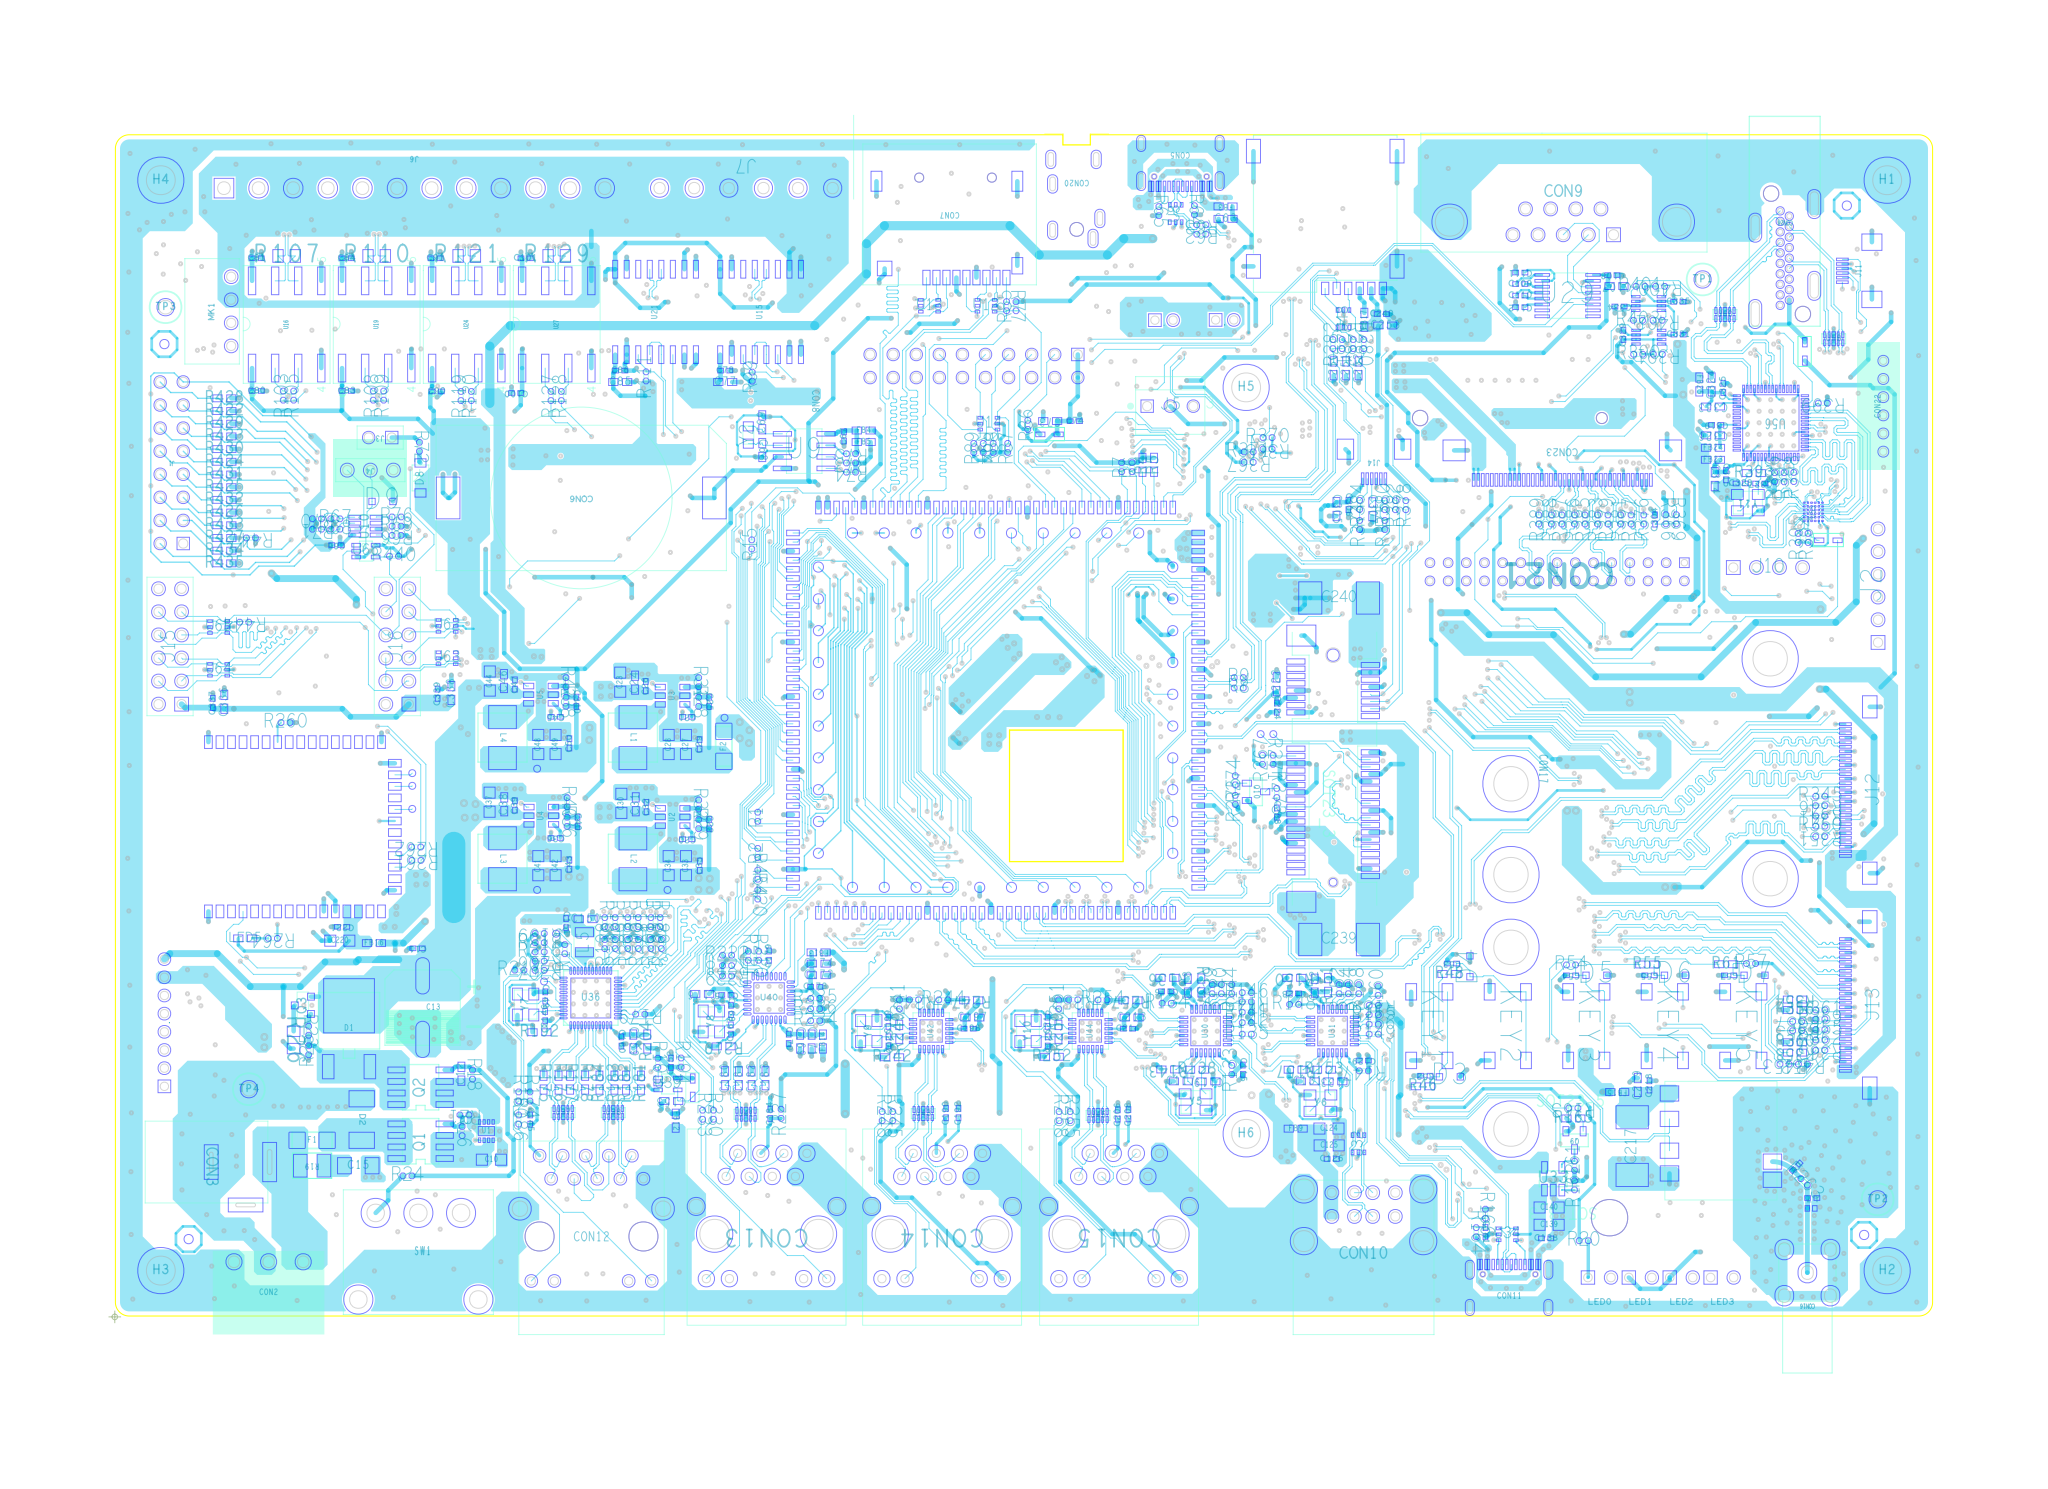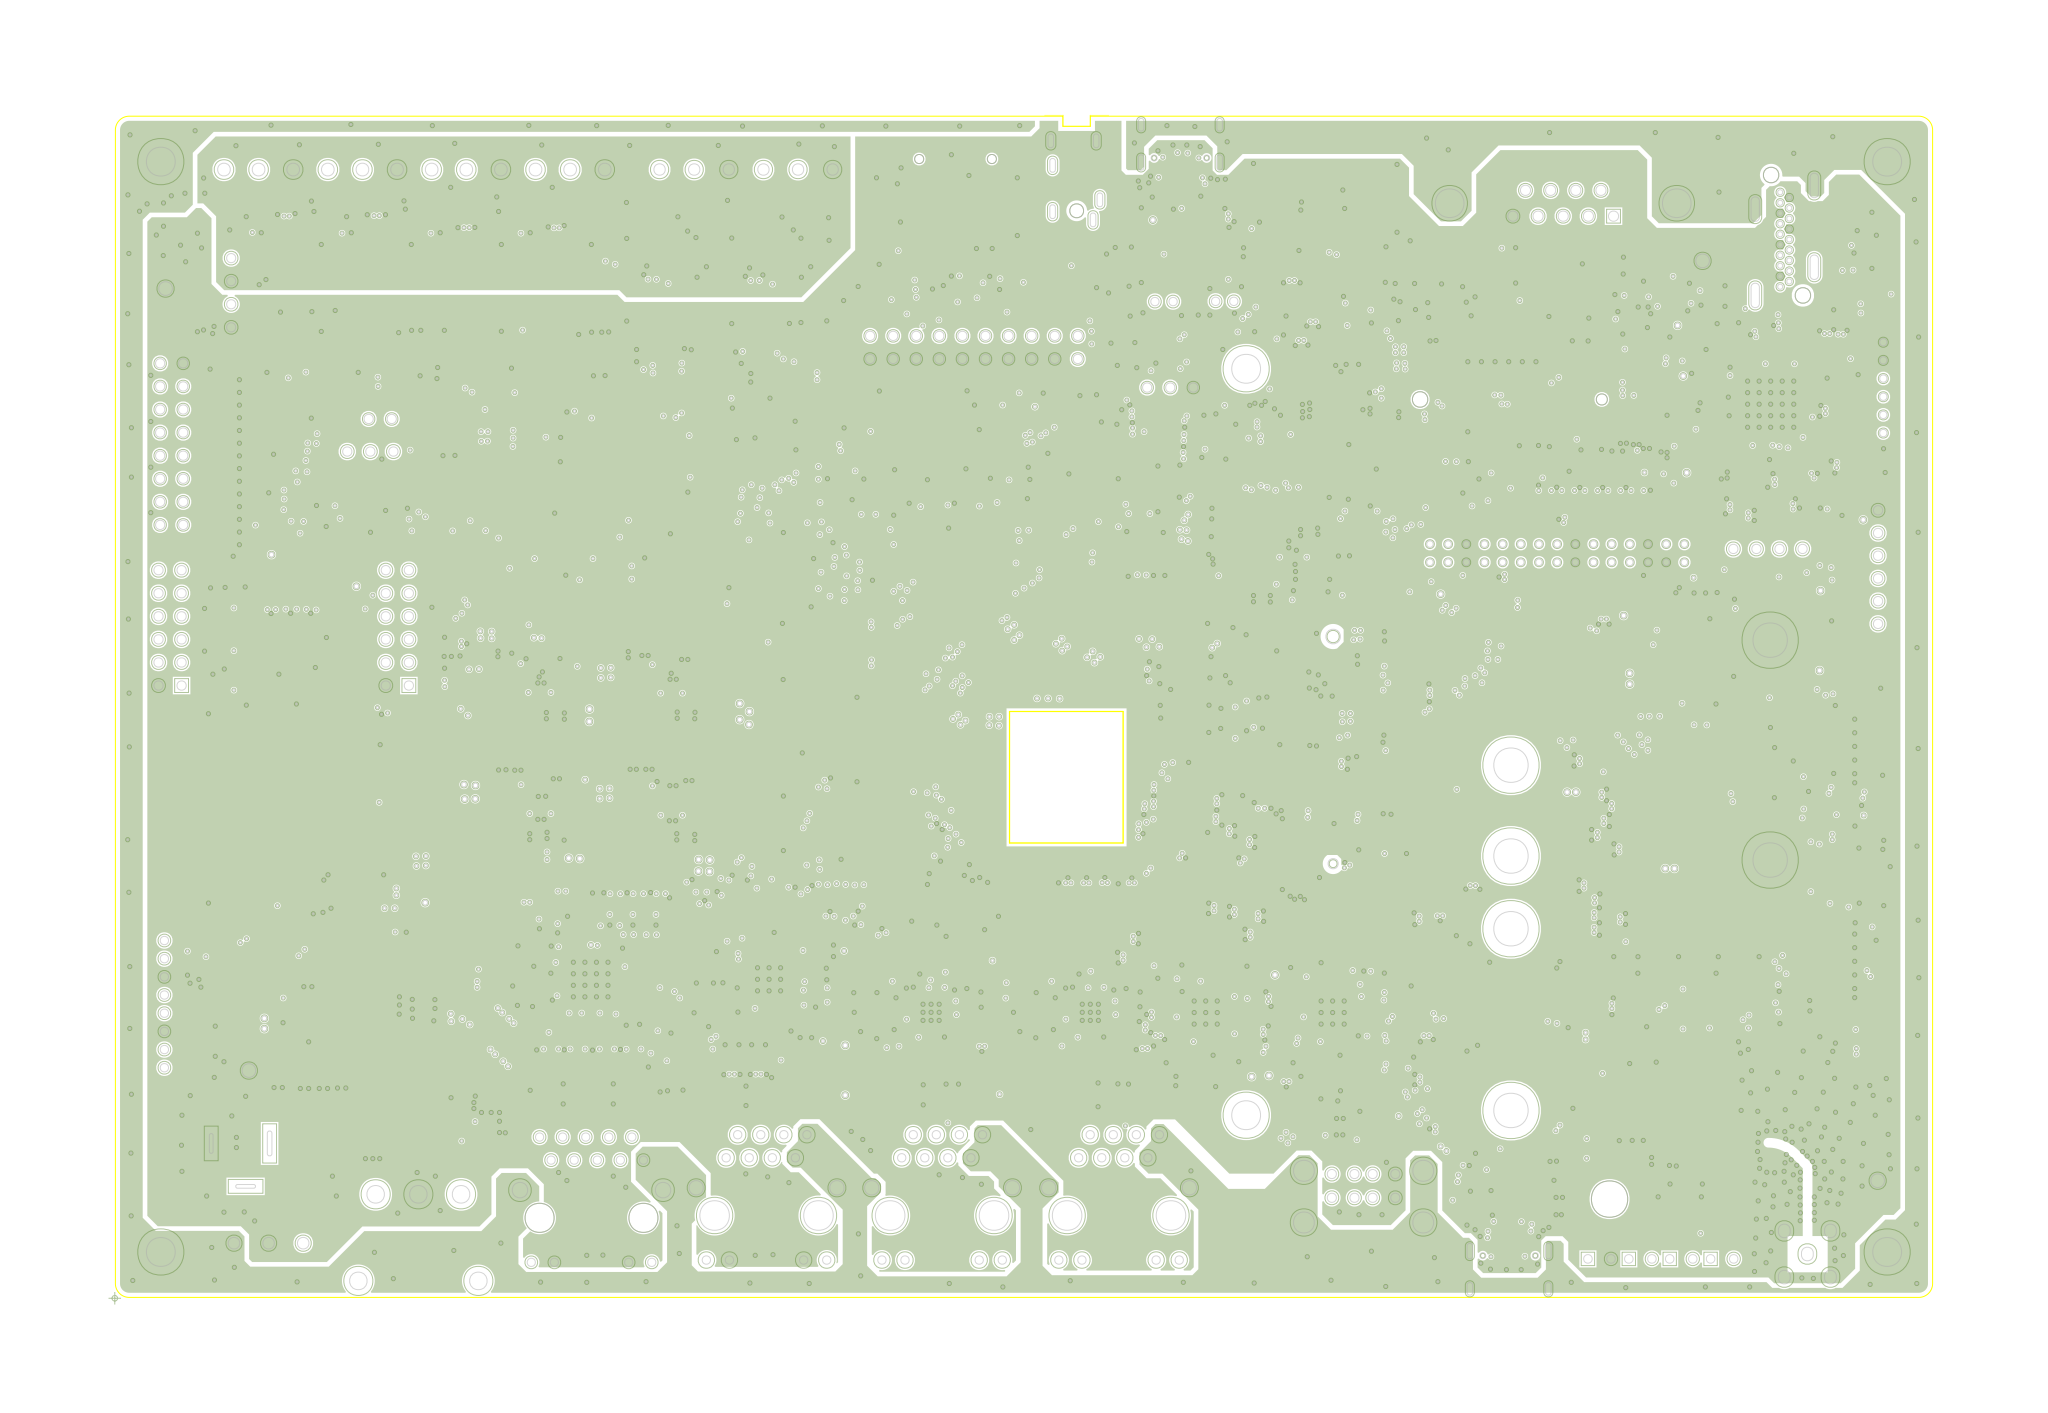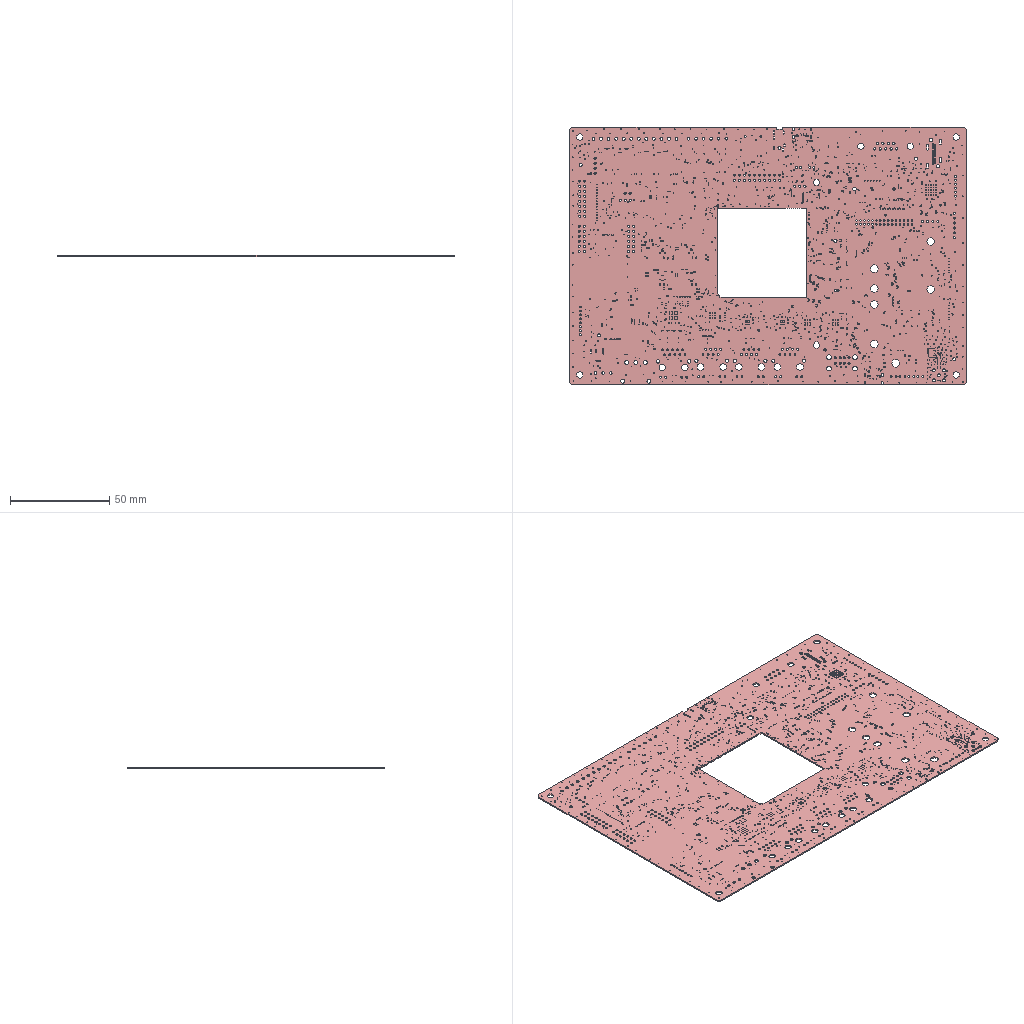Circuit board layout | Cadence Allegro | box 200 x 130 x 0.7 mm
Layer stack:
# Cadence Allegro layer stack of  (unit mm; from the constraint file cross-section; dielectric type: 0 not recorded (Allegro does not mark core vs prepreg), 3 surface material)
index,name,kind,layer,copper_thickness_mm,dielectric_type,dielectric_thickness_mm,dielectric_material,dielectric_constant
0,Top Surface,other,,,,,,
1,TOP,copper,TOP,0.0305,,,,
2,Dielectric1,dielectric,,,0,0.2032,FR-4,4.5
3,GND02,copper,GND02,0.0305,,,,
4,Dielectric2,dielectric,,,0,0.2032,FR-4,4.5
5,VCC03,copper,VCC03,0.0305,,,,
6,Dielectric3,dielectric,,,0,0.2032,FR-4,4.5
7,BOTTOM,copper,BOTTOM,0.0305,,,,
8,Bottom Surface,other,,,,,,
# drill layer pairs: low layer,high layer
drill_pair,TOP,BOTTOM
Part placement, first 484 of 1029 lines:
REFDES,COMP_VALUE,SYM_NAME,SYM_X,SYM_Y,SYM_ROTATE,SYM_MIRROR
C1,680pF_50V,C0603,4512.00,3287.50,180.000,YES
C2,680pF_50V,C0603,4392.00,3287.50,0.000,YES
C3,100nF_25V,C0402,3314.00,3524.00,0.000,YES
C4,100nF_25V,C0402,3314.00,3480.00,0.000,YES
C5,22uF_25V,C0805,4771.35,3338.00,0.000,YES
C6,22uF_25V,C0805,4771.35,3263.00,0.000,YES
C7,100nF_25V,C0402,4707.00,3397.00,180.000,YES
C8,33pF_50V,C0603,3205.00,3430.50,0.000,YES
C9,33pF_50V,C0603,3328.00,3430.50,180.000,YES
C10,22uF_25V,C0805,1590.65,681.00,0.000,NO
C11,100nF_25V,C0402,1312.00,1597.00,180.000,NO
C12,1uF_25V,C0603,1501.88,1053.48,90.000,NO
C13,220uF_35V,CAP_ALU_SMD_8X10D5,1333.90,1340.00,0.000,NO
C14,22pF_50V,C0603,1524.50,805.00,90.000,YES
C15,2.2uF_25V,C1206,1055.00,655.00,0.000,NO
C16,10uF_25V,C0603,364.50,1450.00,90.000,YES
C17,100nF_25V,C0402,315.00,1455.00,90.000,YES
C18,10uF_25V,C0603,316.50,1299.00,270.000,YES
C19,100nF_25V,C0402,366.00,1299.00,270.000,YES
C20,100nF_25V,C0402,2480.00,2070.00,180.000,NO
C21,100nF_25V,C0402,2480.00,2600.00,180.000,NO
C22,15pF_50V,C0402,2575.00,2135.00,270.000,NO
C23,22uF_25V,C0805,2190.00,2708.65,90.000,NO
C24,1uF_25V,C0603,2254.50,2748.00,90.000,NO
C25,15pF_50V,C0402,2575.00,2665.00,270.000,NO
C26,100nF_25V,C0402,2301.00,2733.00,90.000,NO
C27,22uF_25V,C0805,2475.00,2438.65,90.000,NO
C28,22uF_25V,C0805,2400.00,2438.65,90.000,NO
C29,100nF_25V,C0402,2534.00,2481.00,90.000,NO
C30,22uF_25V,C0805,2195.00,2183.65,90.000,NO
C31,1uF_25V,C0603,2257.50,2221.00,90.000,NO
C32,100nF_25V,C0402,2304.00,2209.00,90.000,NO
C33,22uF_25V,C0805,2475.00,1913.66,90.000,NO
C34,22uF_25V,C0805,2400.00,1913.65,90.000,NO
C35,100nF_25V,C0402,2535.00,1955.00,90.000,NO
C36,100nF_25V,C0402,1909.99,2075.00,180.000,NO
C37,22uF_25V,C0805,1623.99,2188.65,90.000,NO
C38,1uF_25V,C0603,1687.49,2221.00,90.000,NO
C39,100nF_25V,C0402,1733.99,2216.00,90.000,NO
C40,15pF_50V,C0402,2004.99,2145.00,270.000,NO
C41,22uF_25V,C0805,1834.99,1913.65,90.000,NO
C42,22uF_25V,C0805,1909.99,1913.65,90.000,NO
C43,100nF_25V,C0402,1969.99,1960.00,90.000,NO
C44,22uF_25V,C0805,1625.00,2713.65,90.000,NO
C45,100nF_25V,C0402,1910.00,2600.00,180.000,NO
C46,1uF_25V,C0603,1686.50,2755.00,90.000,NO
C47,100nF_25V,C0402,1734.00,2740.00,90.000,NO
C48,22uF_25V,C0805,1835.00,2438.65,90.000,NO
C49,22uF_25V,C0805,1910.00,2438.66,90.000,NO
C50,100nF_25V,C0402,1970.00,2485.00,90.000,NO
C51,1nF_2KV,C1210,285.00,4670.00,90.000,YES
C52,10nF_50V,C0402,5679.00,1045.00,180.000,NO
C53,10nF_50V,C0402,5794.00,1531.00,180.000,NO
C54,10nF_50V,C0402,6310.00,1480.00,180.000,NO
C55,10nF_50V,C0402,6650.00,1480.00,180.000,NO
C56,100nF_25V,C0402,7485.00,2935.00,0.000,YES
C57,10nF_50V,C0402,6995.00,1480.00,180.000,NO
C58,100nF_25V,C0402,4884.00,4417.00,180.000,YES
C59,100nF_25V,C0402,4873.00,4640.00,0.000,YES
C60,10nF_50V,C0402,5009.00,4665.00,0.000,YES
C61,10uF_25V,C0603,5035.00,4204.50,180.000,YES
C62,100nF_25V,C0402,5030.00,4255.00,180.000,YES
C63,10uF_25V,C0603,4813.00,4757.50,0.000,NO
C64,22pF_50V,C0603,5289.00,4679.50,180.000,YES
C65,22pF_50V,C0603,5169.00,4679.50,0.000,YES
C66,100nF_25V,C0402,960.00,3344.00,180.000,NO
C67,100nF_25V,C0402,3160.00,3815.00,90.000,NO
C68,DNP_18pF_50V,C0603,2805.50,3756.00,270.000,NO
C69,DNP_18pF_50V,C0603,2805.50,3876.00,90.000,NO
C70,100nF_25V,C0402,3782.00,4479.00,180.000,YES
C71,100nF_25V,C0402,3645.00,4405.00,0.000,YES
C72,10uF_25V,C0603,3640.00,4355.50,0.000,YES
C73,10uF_25V,C0603,4053.00,3881.50,180.000,NO
C74,100nF_25V,C0402,4160.00,3881.00,0.000,NO
C75,100nF_25V,C0402,4745.00,3806.00,270.000,YES
C76,100nF_25V,C0402,4815.00,3832.00,0.000,YES
C77,10uF_25V,C0603,2645.00,4050.50,0.000,NO
C78,100nF_25V,C0402,2645.00,4100.00,0.000,NO
C79,22pF_50V,C0603,2831.00,4464.50,0.000,YES
C80,100nF_25V,C0402,615.00,4011.79,0.000,NO
C81,100nF_25V,C0402,614.77,4586.79,0.000,NO
C82,22pF_50V,C0603,2951.00,4464.50,0.000,YES
C83,100nF_25V,C0402,1005.00,4011.79,0.000,NO
C84,100nF_25V,C0402,1004.77,4586.79,0.000,NO
C85,10uF_25V,C0603,2190.00,4050.50,0.000,NO
C86,100nF_25V,C0402,2190.00,4100.00,0.000,NO
C87,22pF_50V,C0603,2379.00,4464.50,0.000,YES
C88,22pF_50V,C0603,2499.00,4464.50,0.000,YES
C89,100nF_25V,C0402,1911.84,3755.20,180.000,YES
C90,100nF_25V,C0402,1395.00,4010.00,0.000,NO
C91,100nF_25V,C0402,1390.00,4586.79,0.000,NO
C92,15pF_50V,C0402,1367.84,4131.20,270.000,YES
C93,15pF_50V,C0402,1367.84,4046.20,90.000,YES
C94,100nF_25V,C0402,1911.84,3840.20,180.000,YES
C95,100nF_25V,C0402,405.00,4260.00,90.000,YES
C96,10uF_25V,C0603,359.50,4260.00,90.000,YES
C97,100nF_25V,C0402,655.00,4460.00,90.000,YES
C98,10uF_25V,C0603,604.50,4455.00,90.000,YES
C99,100nF_25V,C0402,2673.42,3745.00,180.000,YES
C100,100nF_25V,C0402,1739.00,4003.00,180.000,NO
C101,100nF_25V,C0402,1780.00,4586.79,0.000,NO
C102,15pF_50V,C0402,2124.42,4131.00,270.000,YES
C103,15pF_50V,C0402,2124.42,4046.00,90.000,YES
C104,33pF_50V,C0603,2690.42,4020.50,180.000,YES
C105,33pF_50V,C0603,2690.42,3970.50,180.000,YES
C106,100nF_25V,C0402,2672.42,3834.00,180.000,YES
C107,10uF_25V,C0603,6507.00,4466.50,180.000,NO
C108,100nF_25V,C0402,6489.00,4514.00,180.000,NO
C109,100nF_25V,C0402,6090.00,4475.00,0.000,NO
C110,100nF_25V,C0402,6090.00,4425.00,0.000,NO
C111,100nF_25V,C0402,6090.00,4525.00,180.000,NO
C112,100nF_25V,C0402,6090.00,4375.00,180.000,NO
C113,22uF_25V,C0805,4822.35,1246.00,0.000,YES
C114,100nF_25V,C0402,4799.00,1309.00,0.000,YES
C115,100nF_25V,C0402,4888.00,1071.00,270.000,NO
C116,100nF_25V,C0402,4556.00,1411.00,180.000,NO
C117,DNP_22pF_50V,C0603,4619.00,1020.50,0.000,NO
C118,1uF_25V,C0603,4649.50,1435.00,90.000,NO
C119,DNP_22pF_50V,C0603,4739.00,1020.50,180.000,NO
C120,DNP_100nF_25V,C0402,4656.00,1220.00,180.000,YES
C121,DNP_22uF_25V,C0805,4672.35,1329.00,0.000,YES
C122,DNP_100nF_25V,C0402,4699.00,1158.00,270.000,YES
C123,DNP_100nF_25V,C0402,4656.00,1264.00,180.000,YES
C124,22uF_25V,C0805,5219.65,816.00,0.000,NO
C125,22uF_25V,C0805,5220.65,743.00,0.000,NO
C126,100nF_25V,C0402,5273.00,684.00,0.000,NO
C127,22uF_25V,C0805,5384.35,1242.00,0.000,YES
C128,100nF_25V,C0402,5109.00,1402.00,180.000,NO
C129,100nF_25V,C0402,5412.00,1111.00,180.000,NO
C130,100nF_25V,C0402,5349.00,1309.00,0.000,YES
C131,DNP_22pF_50V,C0603,5169.00,1020.50,0.000,NO
C132,1uF_25V,C0603,5199.50,1435.00,90.000,NO
C133,DNP_22pF_50V,C0603,5289.00,1020.50,180.000,NO
C134,DNP_100nF_25V,C0402,5206.00,1264.00,180.000,YES
C135,DNP_100nF_25V,C0402,5206.00,1220.00,180.000,YES
C136,DNP_100nF_25V,C0402,5249.00,1158.00,270.000,YES
C137,DNP_22uF_25V,C0805,5181.65,1328.00,180.000,YES
C138,100nF_25V,C0402,6202.00,340.00,0.000,NO
C139,22uF_25V,C0805,6173.65,399.00,0.000,NO
C140,22uF_25V,C0805,6173.65,474.00,0.000,NO
C141,100nF_25V,C0402,5939.00,367.00,270.000,NO
C142,100nF_25V,C0402,5922.00,624.00,270.000,YES
C143,100nF_25V,C0402,1886.00,1044.00,0.000,YES
C144,100nF_25V,C0402,2004.00,1044.00,0.000,YES
C145,100nF_25V,C0402,1800.00,855.00,270.000,NO
C146,12pF_50V,C0402,1865.00,1303.34,90.000,NO
C147,100nF_25V,C0402,2242.00,1045.00,180.000,YES
C148,100nF_25V,C0402,2126.00,1044.00,180.000,YES
C149,12pF_50V,C0402,1865.00,1388.34,270.000,NO
C150,4.7uF_25V,C0603,2040.00,1723.16,0.000,NO
C151,100nF_25V,C0402,1955.34,1706.00,270.000,NO
C152,100nF_25V,C0402,2410.00,1101.00,90.000,NO
C153,DNP_1uF_25V,C0603,2411.00,935.50,180.000,NO
C154,100nF_25V,C0402,2066.00,1287.34,270.000,YES
C155,100nF_25V,C0402,2017.00,1287.34,270.000,YES
C156,100nF_25V,C0402,1943.66,1344.00,270.000,YES
C157,1uF_25V,C0603,2241.50,1404.34,90.000,YES
C158,100nF_25V,C0402,2180.00,1408.34,90.000,YES
C159,10uF_25V,C0603,2246.50,1193.34,270.000,NO
C160,100nF_25V,C0402,2195.00,1193.34,270.000,NO
C161,10uF_25V,C0603,2009.50,1470.34,90.000,YES
C162,100nF_25V,C0402,2061.00,1472.34,90.000,YES
C163,10uF_25V,C0603,2170.00,1544.84,180.000,YES
C164,100nF_25V,C0402,2109.00,1472.34,90.000,YES
C165,10uF_25V,C0603,1874.50,1594.34,90.000,YES
C166,100nF_25V,C0402,1945.00,1603.34,90.000,YES
C167,12pF_50V,C0402,2670.00,1245.00,90.000,NO
C168,12pF_50V,C0402,2670.00,1330.00,270.000,NO
C169,10uF_25V,C0603,2969.50,1193.00,270.000,NO
C170,100nF_25V,C0402,2920.00,1205.00,270.000,NO
C171,1uF_25V,C0603,3019.50,1193.00,270.000,NO
C172,10uF_25V,C0603,3050.00,1480.50,0.000,NO
C173,100nF_25V,C0402,3035.00,1430.00,0.000,NO
C174,1uF_25V,C0603,3050.00,1530.50,0.000,NO
C175,100nF_25V,C0402,2650.00,1395.00,180.000,NO
C176,1uF_25V,C0603,2545.00,1399.50,180.000,NO
C177,100nF_25V,C0402,2816.00,1289.00,180.000,YES
C178,1uF_25V,C0603,2745.50,1325.00,270.000,YES
C179,100nF_25V,C0402,2835.00,1565.00,90.000,NO
C180,DNP_15pF_50V,C0603,2644.50,1034.00,90.000,NO
C181,DNP_15pF_50V,C0603,2704.50,1034.00,90.000,NO
C182,DNP_15pF_50V,C0603,2759.50,1034.00,90.000,NO
C183,DNP_15pF_50V,C0603,2819.50,1034.00,90.000,NO
C184,100nF_25V,C0402,2840.00,880.00,90.000,NO
C185,10uF_25V,C0603,3414.50,1425.00,90.000,YES
C186,100nF_25V,C0402,3460.00,1425.00,90.000,YES
C187,100nF_25V,C0402,3473.00,1228.00,90.000,YES
C188,100nF_25V,C0402,3515.00,1158.54,0.000,YES
C189,100nF_25V,C0402,3599.00,1221.54,0.000,YES
C190,100nF_25V,C0402,3602.00,883.00,90.000,NO
C191,100nF_25V,C0402,3590.00,1298.54,90.000,YES
C192,100nF_25V,C0402,3656.00,883.00,90.000,NO
C193,1uF_25V,C0603,3620.00,1164.04,0.000,YES
C194,100nF_25V,C0402,3520.00,1297.54,90.000,YES
C195,1uF_25V,C0603,3720.50,1313.54,270.000,YES
C196,100nF_25V,C0402,3667.00,1315.54,270.000,YES
C197,1uF_25V,C0603,3716.00,1297.04,0.000,NO
C198,100nF_25V,C0402,3700.00,1248.54,0.000,NO
C199,12pF_50V,C0402,3352.00,1278.54,90.000,NO
C200,12pF_50V,C0402,3352.00,1193.54,270.000,NO
C201,10uF_25V,C0603,4104.50,1425.00,90.000,YES
C202,100nF_25V,C0402,4150.00,1425.00,90.000,YES
C203,100nF_25V,C0402,4163.00,1228.00,90.000,YES
C204,100nF_25V,C0402,4205.00,1158.54,0.000,YES
C205,100nF_25V,C0402,4289.00,1221.54,0.000,YES
C206,100nF_25V,C0402,4346.44,877.00,90.000,NO
C207,100nF_25V,C0402,4280.00,1298.54,90.000,YES
C208,100nF_25V,C0402,4392.44,878.00,90.000,NO
C209,1uF_25V,C0603,4310.00,1164.04,0.000,YES
C210,100nF_25V,C0402,4210.00,1297.54,90.000,YES
C211,1uF_25V,C0603,4410.50,1318.54,270.000,YES
C212,100nF_25V,C0402,4357.00,1315.54,270.000,YES
C213,1uF_25V,C0603,4406.00,1297.04,0.000,NO
C214,100nF_25V,C0402,4390.00,1248.54,0.000,NO
C215,12pF_50V,C0402,4042.00,1278.54,90.000,NO
C216,12pF_50V,C0402,4042.00,1193.54,270.000,NO
C217,220uF_10V,CAP_CASE_D,6575.00,740.00,90.000,NO
C218,100nF_25V,C0402,6650.00,1003.00,90.000,NO
C219,10uF_25V,C0603,6599.50,1005.00,90.000,NO
C220,22uF_25V,C0805,933.65,1630.00,0.000,NO
C221,100nF_25V,C0402,985.00,1690.00,180.000,NO
C222,10uF_25V,C0603,5034.50,2741.00,90.000,NO
C223,47pF_50V,C0603,5450.00,2795.50,180.000,YES
C224,100nF_25V,C0402,5035.00,2640.00,270.000,NO
C225,100nF_25V,C0402,5443.00,2750.00,180.000,YES
C226,22uF_25V,C0805,5214.65,2093.00,180.000,YES
C227,100nF_25V,C0402,5116.00,2068.00,0.000,YES
C228,10nF_50V,C0402,5549.00,1927.00,180.000,YES
C229,100nF_25V,C0402,5450.00,2888.00,180.000,YES
C230,100pF_50V,C0603,5533.50,2432.00,270.000,YES
C231,100nF_25V,C0402,5450.00,2845.00,180.000,YES
C232,12pF_50V,C0402,5442.00,1927.00,0.000,YES
C233,100nF_25V,C0402,4927.00,2855.00,270.000,YES
C234,10uF_25V,C0603,4872.50,2865.00,270.000,YES
C235,10uF_25V,C0603,5226.50,2544.00,270.000,YES
C236,100nF_25V,C0402,5276.00,2544.00,270.000,YES
C237,1uF_25V,C0603,5131.50,2747.00,90.000,YES
C238,100nF_25V,C0402,5035.00,2185.00,270.000,NO
C239,220uF_10V,CAP_CASE_D,5305.00,1635.00,0.000,NO
C240,220uF_10V,CAP_CASE_D,5305.00,3115.00,0.000,NO
C241,100nF_25V,C0402,5463.00,2379.00,270.000,YES
C242,12pF_50V,C0402,5116.00,2113.00,0.000,YES
C243,100nF_25V,C0402,6672.00,3633.00,90.000,YES
C244,10pF_25V,C0603,6679.50,3760.00,90.000,YES
C245,33pF_50V,C0603,6579.50,3760.00,90.000,YES
C246,100nF_25V,C0402,6530.00,3755.00,90.000,YES
C247,10uF_25V,C0603,6629.50,3760.00,90.000,YES
C248,220uF_10V,CAP_CASE_D,6620.00,4105.00,90.000,YES
C249,10nF_50V,C0402,5490.00,4345.00,0.000,NO
C250,DNP_33pF_50V,C0603,5281.50,4110.00,90.000,NO
C251,DNP_33pF_50V,C0603,5335.50,4110.00,90.000,NO
C252,DNP_33pF_50V,C0603,5389.50,4110.00,90.000,NO
C253,1uF_25V,C0603,5505.00,4295.50,0.000,NO
C254,100nF_25V,C0402,5971.22,4235.00,270.000,YES
C255,100nF_25V,C0402,5931.22,4235.00,270.000,YES
C256,100nF_25V,C0402,5865.00,3671.00,270.000,YES
C257,100nF_25V,C0402,5636.00,4235.00,270.000,YES
C258,10pF_25V,C0603,5415.50,3775.00,270.000,YES
C259,33pF_50V,C0603,5515.50,3775.00,270.000,YES
C260,100nF_25V,C0402,5560.00,3765.00,270.000,YES
C261,10uF_25V,C0603,5465.50,3775.00,270.000,YES
C262,220uF_10V,CAP_CASE_D,5350.00,3405.00,270.000,YES
C263,100nF_25V,C0402,5185.00,3235.00,0.000,YES
C264,22uF_25V,C0805,4897.00,3112.35,90.000,YES
C265,1uF_25V,C0603,4960.50,3078.00,90.000,YES
C266,100nF_25V,C0402,5007.00,3093.00,90.000,YES
C267,15pF_50V,C0402,5275.00,3165.00,270.000,YES
C268,22uF_25V,C0805,5099.00,3399.35,90.000,YES
C269,22uF_25V,C0805,5174.00,3399.34,90.000,YES
C270,100nF_25V,C0402,5234.00,3358.00,90.000,YES
C271,22uF_10V,C0603,4575.00,4062.50,0.000,YES
C272,100pF_50V,C0603,4515.00,4162.50,0.000,YES
C273,10uF_25V,C0603,7016.50,2627.00,270.000,YES
C274,100nF_25V,C0402,6993.00,3009.00,270.000,YES
C275,100nF_25V,C0402,6743.00,3009.00,270.000,YES
C276,100nF_25V,C0402,6963.00,2579.00,90.000,YES
C277,10uF_25V,C0603,6654.00,3101.50,0.000,YES
C278,100nF_25V,C0402,6759.00,3101.00,180.000,YES
C279,10nF_50V,C0402,6913.00,2579.00,90.000,YES
C280,10nF_50V,C0402,6893.00,3009.00,270.000,YES
C281,10nF_50V,C0402,6793.00,3009.00,270.000,YES
C282,10nF_50V,C0402,6943.00,3009.00,270.000,YES
C283,10nF_50V,C0402,6843.00,3009.00,270.000,YES
C284,10uF_25V,C0603,7641.00,3607.50,180.000,YES
C285,100nF_25V,C0402,7644.00,3655.00,180.000,YES
C286,10uF_25V,C0603,7605.50,4579.00,270.000,YES
C287,100nF_25V,C0402,7560.00,4579.00,270.000,YES
C288,100nF_25V,C0402,7543.88,2115.05,270.000,YES
C289,10uF_25V,C0603,7495.05,1950.62,180.000,YES
C290,100nF_25V,C0402,7495.05,2001.12,180.000,YES
C291,100nF_25V,C0402,7633.00,1965.00,90.000,YES
C292,100nF_25V,C0402,7665.00,2215.00,270.000,YES
C293,100nF_25V,C0402,7645.00,1600.00,90.000,YES
C294,100nF_25V,C0402,7665.00,1850.00,270.000,YES
C295,100nF_25V,C0402,7408.00,1165.00,0.000,YES
C296,10uF_25V,C0603,7484.00,1021.50,0.000,YES
C297,100nF_25V,C0402,7491.00,1070.00,0.000,YES
C298,100nF_25V,C0402,5020.00,3796.00,270.000,YES
C299,10uF_25V,C0603,4923.50,3806.00,270.000,YES
C300,10uF_25V,C0603,4975.50,3806.00,270.000,YES
C301,1uF_25V,C0603,5280.00,3930.50,0.000,YES
C302,10uF_25V,C0603,6754.62,3622.03,270.000,YES
C303,100nF_25V,C0402,6623.00,3633.00,270.000,YES
C304,100nF_25V,C0402,6674.00,3455.00,90.000,NO
C305,10uF_25V,C0603,5293.50,3500.00,270.000,NO
C306,100nF_25V,C0402,5345.00,3518.00,270.000,NO
C307,1uF_25V,C0603,5448.50,3499.00,270.000,NO
C308,10uF_25V,C0603,6931.00,4007.50,0.000,YES
C309,100nF_25V,C0402,7032.00,3971.00,180.000,YES
C310,100nF_25V,C0402,7192.00,3745.00,270.000,YES
C311,100nF_25V,C0402,7238.00,4018.00,0.000,YES
C312,10uF_25V,C0603,7295.00,3848.50,0.000,YES
C313,100nF_25V,C0402,7303.00,3802.00,0.000,YES
C314,10uF_25V,C0603,6932.50,3630.00,270.000,NO
C315,100nF_25V,C0402,6981.00,3647.00,270.000,NO
C316,10uF_25V,C0603,6930.00,3849.50,180.000,YES
C317,10uF_25V,C0603,6930.00,3904.50,180.000,YES
C318,100nF_25V,C0402,6930.00,3805.00,180.000,YES
C319,100nF_25V,C0402,6939.00,3865.00,180.000,NO
C320,10uF_25V,C0603,7030.50,3757.00,270.000,YES
C321,100nF_25V,C0402,7103.00,3747.00,270.000,YES
C322,10uF_25V,C0603,7098.50,4012.00,90.000,YES
C323,100nF_25V,C0402,7148.00,3999.00,90.000,YES
C324,10uF_25V,C0603,6919.50,4040.00,90.000,NO
C325,100nF_25V,C0402,6970.00,4025.00,90.000,NO
C326,10uF_25V,C0603,6925.00,3819.50,180.000,NO
C327,12pF_50V,C0402,7130.00,3611.00,180.000,NO
C328,12pF_50V,C0402,7045.00,3611.00,0.000,NO
C329,100nF_25V,C0402,6537.00,4255.00,90.000,NO
C330,100nF_25V,C0402,7395.00,3778.00,270.000,YES
C331,100nF_25V,C0402,6776.00,4256.00,0.000,NO
C332,100nF_25V,C0402,7473.00,3420.00,180.000,YES
C333,2.2nF_50V,C0603,6925.00,3944.50,180.000,NO
C334,100nF_25V,C0402,6520.00,4378.00,180.000,NO
C335,100nF_25V,C0402,6775.00,4398.00,0.000,NO
C336,10uF_25V,C0603,474.50,2665.00,90.000,NO
C337,100nF_25V,C0402,425.00,2660.00,90.000,NO
C338,10uF_25V,C0603,1458.50,2703.00,90.000,NO
C339,100nF_25V,C0402,1399.00,2700.00,90.000,NO
C340,15pF_50V,C0402,2000.00,2665.00,270.000,NO
C341,22uF_25V,C0805,1391.00,2743.35,90.000,YES
C342,22uF_25V,C0805,1474.00,2741.35,90.000,YES
CON0,SMD_200PIN_TL3562,SMD_200P_45X45_TL3562,3816.51,2628.84,0.000,NO
CON2,CON_3P_3D81_90_MALE,CON_3P_3D81_90_MALE_NEW,816.48,238.72,0.000,NO
CON3,305-OT03SZD001,CON_DC005_NEW,434.90,670.87,270.000,NO
CON4,CON_2D0MM_8P,DIP_CON_2D0MM_8P,214.89,1274.54,270.000,NO
CON5,KH-TYPE-C-16P,TYPE-C_16P_90_SMD,4617.31,5038.28,180.000,NO
CON6,CR2032-BS-6-1,CON_BATTERY_CR2032,2021.16,3548.39,180.000,NO
CON7,1060802AR013,CON_TF_CARD,3642.94,4936.30,180.000,NO
CON8,IDC_20P,CON_2D54_2X10_TH_BOX_90,4172.84,4070.00,270.000,NO
CON9,D-DMR009PM-D002,CON_DB9,6276.09,4688.68,0.000,NO
CON10,FUS208-FDBW3K,CON_USBA_DUAL,5411.03,328.35,0.000,NO
CON11,KH-TYPE-C-16P,TYPE-C_16P_90_SMD,6041.51,87.18,0.000,NO
CON12,KRJ-320DNL,KRJ-320DNL_14P,2065.66,348.52,0.000,NO
CON13,KRJ-138EHNL,CON_YDS_13F-64GYD2PLXNL,2824.08,643.62,180.000,NO
CON14,KRJ-138EHNL,CON_YDS_13F-64GYD2PLXNL,3584.76,643.62,180.000,NO
CON15,KRJ-138EHNL,CON_YDS_13F-64GYD2PLXNL,4351.44,643.62,180.000,NO
CON16,KH-SMA-K513-G,CON_SMA_5P_V_DIP,7334.01,191.79,180.000,NO
CON17,KH-PCIE5.2H-52P,CON_MINI_PCIE_4G,5279.14,2375.14,270.000,NO
CON18,SI63C-01200,MICRO-SIM,5246.93,4792.23,180.000,NO
CON19,CON_M_2,CONN-SMD_APCI0103-P001A,6049.67,3953.56,0.000,YES
CON20,JQ-PJ-3106A-1,PJ-342E,4167.90,5125.36,180.000,NO
CON21,PZ200-2-15-Z-2.0-G0,CON_2MM_2X15P,6249.86,3228.32,180.000,NO
CON22,A2001WV-6P-3,CON_PHD_2D0_1X6P_TH_180,7663.07,3945.70,90.000,NO
CON23,FFC_0.5mm_40P_DOWN,CON_FFC_0D5_40P,6656.10,3626.46,180.000,NO
CON24,FHD14-FDB300K6K,DIP_HDMI-A,7235.95,4746.88,180.000,NO
D1,MBR1060CD,TO-252,1015.00,1216.10,0.000,NO
D2,SMBJ16CA,SMB,1070.00,855.00,270.000,NO
D3,LC05CI,SOD323_BI,5785.00,1040.10,0.000,NO
D4,LC05CI,SOD323_BI,5871.90,1519.00,90.000,NO
D5,LC05CI,SOD323_BI,6420.00,1480.10,0.000,NO
D6,LC05CI,SOD323_BI,6760.00,1480.10,0.000,NO
D7,LC05CI,SOD323_BI,7105.00,1480.10,0.000,NO
D8,SD103AW,SOD-123_NEW,1324.50,3635.00,90.000,NO
D9,LC05CI,SOD323_BI,1160.00,3533.10,0.000,NO
D10,B5819WS-SL,SOD-323,6046.20,531.00,90.000,YES
D11,B5819WS-SL,SOD-323,2504.20,993.00,90.000,NO
D12,PESD2442U005,ESD_0402,7350.00,470.00,0.000,NO
D13,LC05CI,SOD323_BI,4870.00,4216.90,180.000,YES
D14,LC05CI,SOD323_BI,4740.00,4217.10,0.000,YES
D15,LC05CI,SOD323_BI,4585.00,4216.90,180.000,YES
D16,LC05CI,SOD323_BI,4445.00,4217.10,0.000,YES
D17,LC05CI,SOD323_BI,4334.90,4570.00,90.000,YES
D18,LC05CI,SOD323_BI,4404.90,4570.00,90.000,YES
D19,SS14,SMA,5285.00,3760.00,270.000,YES
D20,B5819WS-SL,SOD-323,7323.20,4183.00,90.000,NO
D21,B5819WS-SL,SOD-323,7382.20,3671.00,90.000,YES
D22,B5819WS-SL,SOD-323,7425.00,3364.80,0.000,NO
D23,LC05CI,SOD323_BI,390.00,1150.90,180.000,YES
D24,LC05CI,SOD323_BI,390.00,1075.90,180.000,YES
D25,B5819WS-SL,SOD-323,4050.00,3823.80,0.000,NO
F1,FUSE 2A,F1206,855.00,765.00,0.000,NO
F2,FUSE 3A,F1206,2639.00,2472.00,90.000,NO
FB1,220R_100MHz_2A,L0603,4472.50,3200.00,270.000,YES
FB2,220R_100MHz_2A,L0603,4420.50,3200.00,270.000,YES
FB3,220R_100MHz_2A,L0603,4813.00,4811.50,180.000,NO
FB4,220R_100MHz_2A,L0603,3245.00,3840.50,0.000,NO
FB5,DNP_220R_100MHz_2A,L0603,3245.00,3790.50,0.000,NO
FB6,220R_100MHz_2A,L0603,4697.50,3737.00,270.000,YES
FB7,220R_100MHz_2A,L0603,4887.50,1221.00,270.000,YES
FB8,DNP_220R_100MHz_2A,L0603,4804.00,1360.50,180.000,YES
FB9,220R_100MHz_2A,L0603,5117.00,815.50,0.000,NO
FB10,220R_100MHz_2A,L0603,5449.50,1258.00,270.000,YES
FB11,DNP_220R_100MHz_2A,L0603,5327.00,1389.50,180.000,YES
FB12,220R_100MHz_2A,L0603,2430.50,850.00,270.000,NO
FB13,220R_100MHz_2A,L0603,3050.00,1579.50,180.000,NO
FB14,220R_100MHz_2A,L0603,3068.50,1193.00,90.000,NO
FB15,220R_100MHz_2A,L0603,6510.00,974.50,180.000,NO
FB16,220R_100MHz_2A,L0603,1123.00,1619.50,0.000,NO
FB17,DNP_220R_100MHz_2A,L0603,5414.50,4320.00,90.000,NO
FB18,220R_100MHz_2A,L0603,6686.50,3004.00,90.000,YES
FB19,DNP_220R_100MHz_2A,L0603,6626.50,3004.00,90.000,YES
FB20,220R_100MHz_2A,L0603,6931.00,3955.50,180.000,YES
FB21,220R_100MHz_2A,L0603,7324.50,3937.00,90.000,YES
FB22,220R_100MHz_2A,L0603,6945.00,3757.50,180.000,YES
FB23,220R_100MHz_2A,L0603,6925.00,3713.50,0.000,NO
FB24,220R_100MHz_2A,L0603,6925.00,3765.50,0.000,NO
FB25,220R_100MHz_2A,L0603,6865.50,4040.00,270.000,NO
FB26,220R_100MHz_2A,L0603,6931.00,4061.50,180.000,YES
FB27,DNP_220R_100MHz_2A,L0603,7405.50,3347.00,270.000,YES
FB28,220R_100MHz_2A,L0603,7457.50,3504.00,90.000,YES
H1,HOLE,MHOLE_C200D125,7679.78,4925.02,0.000,NO
H2,HOLE,MHOLE_C200D125,7679.78,200.61,0.000,NO
H3,HOLE,MHOLE_C200D125,199.47,200.61,0.000,NO
H4,HOLE,MHOLE_C200D125,199.47,4925.02,0.000,NO
H5,HOLE,MHOLE_C200D125,4902.20,4027.40,0.000,NO
H6,HOLE,MHOLE_C200D125,4902.20,793.20,0.000,NO
H7,HOLE,NHOLE_C4_BT,6476.90,429.78,0.000,NO
H8,HOLE,5G_HOLE_3D5,6049.67,1916.21,90.000,YES
J1,PZ254-2-08-Z-8.5-G0,CON_2D54_2X8_TH,246.60,3950.93,180.000,NO
J2,A2501WV-06A,CON_XH_1X6P_2D54_H_M_DIP,7640.24,2922.19,90.000,NO
J3,KH-2.54PH180-1X2P-L11.5,HEADER_1X2P_2D54_MALE,1200.00,3810.00,180.000,NO
J4,KH-2.54PH180-1X3P-L11.5,CON3_2D254,1207.36,3668.83,180.000,NO
J5,FWF25401-S03S22W5B,MOL22-23-2031,4473.35,3946.09,0.000,NO
J6,KF2EDGR-3.81-12P,KF2EDGR-3D81-12P,473.08,4890.67,180.000,NO
J7,KF2EDGR-3.81-06P,KF2EG_3_81-6P,2738.58,4892.86,180.000,NO
J8,CN2M_2R00_V_P_DIP,CN2M_2R00_V_P_DIP,4809.35,4319.64,180.000,NO
J9,CN2M_2R00_V_P_DIP,CN2M_2R00_V_P_DIP,4546.35,4318.65,180.000,NO
J10,KH-2.54PH180-1X4P-L11.5,CON_TH_1X4P_2D54_H_DIP,7013.23,3246.86,0.000,NO
J11,11203-06010-11,CON_FFC_0D5_6P,7485.67,4483.36,90.000,NO
J12,11203-30010-11,CON_FFC_0D5_30P,7498.84,1997.33,90.000,NO
J13,11203-30010-11,CON_FFC_0D5_30P,7498.79,1066.21,90.000,NO
J14,11203-06010-11,CON_FFC_0D5_6P,5505.50,3631.64,180.000,NO
J15,2.54MM 2x6P TH FEMALE,HEADER_2X6_2D54_MALE,289.46,2654.86,90.000,NO
J16,2.54MM 2x6P TH FEMALE,HEADER_2X6_2D54_MALE,1274.26,2654.86,90.000,NO
KEY1,TS-1158B-B-B-W,TS-1158B-B-B-W,5695.88,1259.81,270.000,NO
KEY2,TS-1158B-B-B-W,TS-1158B-B-B-W,6036.03,1259.81,270.000,NO
KEY3,TS-1158B-B-B-W,TS-1158B-B-B-W,6376.16,1259.81,270.000,NO
KEY4,TS-1158B-B-B-W,TS-1158B-B-B-W,6716.30,1259.81,270.000,NO
KEY5,TS-1158B-B-B-W,TS-1158B-B-B-W,7056.44,1259.81,270.000,NO
L1,CSAB0518-2R2M,SMD_CSAB0518,2245.00,2509.99,270.000,NO
L2,CSAB0518-2R2M,SMD_CSAB0518,2245.00,1985.00,270.000,NO
L3,CSAB0518-2R2M,SMD_CSAB0518,1680.00,1985.00,270.000,NO
L4,CSAB0518-2R2M,SMD_CSAB0518,1680.00,2509.99,270.000,NO
L5,2.2uH_2.4A,SMD-L2520M-2P,2035.00,1623.34,90.000,NO
L6,DNP_5.6nH_300mA,L0402,7285.00,650.00,225.000,NO
L7,DNP_5.6nH_300mA,L0402,7355.00,515.00,180.000,NO
L8,CSAB0518-2R2M,SMD_CSAB0518,4949.00,3314.00,270.000,YES
L9,PRS4018-150MT,L_L4D5XW4D0_H3D2,5094.60,3653.80,90.000,YES
LED0,RED_LED,CON_2P_3MM,6383.16,170.60,0.000,NO
LED1,GREEN_LED,CON_2P_3MM,6560.32,170.60,0.000,NO
LED2,GREEN_LED,CON_2P_3MM,6737.49,170.60,0.000,NO
LED3,YELLOW_LED,CON_2P_3MM,6914.66,170.60,0.000,NO
LED4,LED_GREEN,D0603,6757.00,3770.00,90.000,YES
LED5,LED_GREEN,D0603,565.00,1640.00,0.000,NO
MK1,B0505S-1WR3L,DIP4_B0505S_1W,403.95,4356.97,90.000,NO
MK2,WH-BLE105,SMD_44P_1822X2680_WH-BLE105,405.71,1756.95,90.000,NO
Q1,WPM3021-8/TR,PSOPSOP-8L,1325.32,761.17,90.000,NO
Q2,WPM3021-8/TR,PSOPSOP-8L,1325.00,995.00,90.000,NO
Q3,CJ3401,SOT23-3,815.00,1350.00,180.000,NO
Q4,CJ3401,SOT23-3,1964.99,1985.00,270.000,YES
Q5,MMBT3904,SOT23-3_DBZ3,6675.00,400.00,180.000,YES
Q6,MMBT3904,SOT23-3_DBZ3,6810.00,400.00,180.000,YES
Q7,CJ3401,SOT23-3,4822.00,3746.50,180.000,YES
Q8,MMBT3904,SOT23-3_DBZ3,4820.00,3591.00,270.000,YES
Q9,MMBT3904,SOT23-3_DBZ3,6325.00,765.00,180.000,NO
Q10,MMBT3904,SOT23-3_DBZ3,4945.00,2275.00,270.000,NO
Q11,CJ3400,SOT23-3_DBZ3,6990.00,400.00,180.000,YES
Q12,CJ3400,SOT23-3_DBZ3,5966.00,3626.00,0.000,YES
Q13,CJ3400,SOT23-3_DBZ3,5455.00,4280.00,0.000,YES
Q14,MMBT3904,SOT23-3_DBZ3,6755.00,4390.00,90.000,YES
Q15,CJ3401,SOT23-3,3330.00,1410.00,180.000,YES
Q16,CJ3401,SOT23-3,4020.00,1410.00,180.000,YES
Pad and via stacks, first 108 of 196 lines:
# Allegro (Cadence) via spans and padstacks; design units: ("mils" 2 100)
# via spans: padstack,start_layer,end_layer,net_example,count
# Allegro padstack definitions: name,start_layer,end_layer,drill,plating,holeType,type
SMD40X30,"ETCH/TOP","ETCH/TOP",0.0,"PLATED","none","smd"
SMD25X20,"ETCH/TOP","ETCH/TOP",0.0,"PLATED","none","smd"
S48,"ETCH/TOP","ETCH/TOP",0.0,"PLATED","none","smd"
OB15X40,"ETCH/TOP","ETCH/TOP",0.0,"PLATED","none","smd"
SMD100X140,"ETCH/TOP","ETCH/TOP",0.0,"PLATED","none","smd"
SMD60X70,"ETCH/TOP","ETCH/TOP",0.0,"PLATED","none","smd"
SMD11_35V,"ETCH/TOP","ETCH/TOP",0.0,"NON_PLATED","none","smd"
SMD11_31V,"ETCH/TOP","ETCH/TOP",0.0,"NON_PLATED","none","smd"
SMD_R610X118P0S40,"ETCH/TOP","ETCH/TOP",0.0,"PLATED","none","smd"
SMD_R1083X472P0S40,"ETCH/TOP","ETCH/TOP",0.0,"PLATED","none","smd"
PAD062X104,"ETCH/TOP","ETCH/TOP",0.0,"NON_PLATED","none","smd"
PAD032X054,"ETCH/TOP","ETCH/TOP",0.0,"NON_PLATED","none","smd"
SMD96X90,"ETCH/TOP","ETCH/TOP",0.0,"PLATED","none","smd"
SMD55X12,"ETCH/TOP","ETCH/TOP",0.0,"PLATED","none","smd"
SMD11_45V,"ETCH/TOP","ETCH/TOP",0.0,"PLATED","none","smd"
SMD46X26,"ETCH/TOP","ETCH/TOP",0.0,"PLATED","none","smd"
SMD_0D8X1D6_REC,"ETCH/TOP","ETCH/TOP",0.0,"PLATED","none","smd"
SMD_2D2X1D2_REC_1,"ETCH/TOP","ETCH/TOP",0.0,"PLATED","none","smd"
SMD_1D8X1D2_REC_1,"ETCH/TOP","ETCH/TOP",0.0,"PLATED","none","smd"
SMD_1D6_SQU_1,"ETCH/TOP","ETCH/TOP",0.0,"PLATED","none","smd"
SMD220_235-NP,"ETCH/TOP","ETCH/TOP",0.0,"PLATED","none","smd"
SMD50_105,"ETCH/TOP","ETCH/TOP",0.0,"PLATED","none","smd"
SMD70X110,"ETCH/TOP","ETCH/TOP",0.0,"PLATED","none","smd"
SMD07X07,"ETCH/TOP","ETCH/TOP",0.0,"PLATED","none","smd"
SMD20_24,"ETCH/TOP","ETCH/TOP",0.0,"PLATED","none","smd"
SMD80_80,"ETCH/TOP","ETCH/TOP",0.0,"PLATED","none","smd"
36X48,"ETCH/TOP","ETCH/TOP",0.0,"PLATED","none","smd"
RX1_80Y1_80R0_10T,"ETCH/TOP","ETCH/TOP",0.0,"PLATED","none","smd"
SMD96_63H,"ETCH/TOP","ETCH/TOP",0.0,"PLATED","none","smd"
SMD51X12,"ETCH/TOP","ETCH/TOP",0.0,"PLATED","none","smd"
SMD11_51V,"ETCH/TOP","ETCH/TOP",0.0,"PLATED","none","smd"
SMD71_87V,"ETCH/TOP","ETCH/TOP",0.0,"PLATED","none","smd"
SMD81_55H,"ETCH/TOP","ETCH/TOP",0.0,"PLATED","none","smd"
SMD100_120,"ETCH/TOP","ETCH/TOP",0.0,"PLATED","none","smd"
SMD157_83H,"ETCH/TOP","ETCH/TOP",0.0,"PLATED","none","smd"
040X080V,"ETCH/TOP","ETCH/TOP",0.0,"PLATED","none","smd"
SMD25_75,"ETCH/TOP","ETCH/TOP",0.0,"PLATED","none","smd"
SMD25X6_40,"ETCH/TOP","ETCH/TOP",0.0,"PLATED","none","smd"
SMD30X30,"ETCH/TOP","ETCH/TOP",0.0,"PLATED","none","smd"
SMD0R635-OT,"ETCH/TOP","ETCH/TOP",0.0,"PLATED","none","smd"
SMD45X55,"ETCH/TOP","ETCH/TOP",0.0,"PLATED","none","smd"
C30,"ETCH/TOP","ETCH/TOP",0.0,"PLATED","none","smd"
SMD70_40,"ETCH/TOP","ETCH/TOP",0.0,"PLATED","none","smd"
SMD10_20,"ETCH/TOP","ETCH/TOP",0.0,"PLATED","none","smd"
SMD16X52,"ETCH/TOP","ETCH/TOP",0.0,"NON_PLATED","none","smd"
CD50X30,"ETCH/TOP","ETCH/TOP",0.0,"PLATED","none","smd"
SMD65REC13,"ETCH/TOP","ETCH/TOP",0.0,"PLATED","none","smd"
22X77REC,"ETCH/TOP","ETCH/TOP",0.0,"PLATED","none","smd"
SMD37REC16MM_1,"ETCH/TOP","ETCH/TOP",0.0,"PLATED","none","smd"
SMD24_44V,"ETCH/TOP","ETCH/TOP",0.0,"PLATED","none","smd"
CD160X30,"ETCH/TOP","ETCH/TOP",0.0,"PLATED","none","smd"
SMD35_10H,"ETCH/TOP","ETCH/TOP",0.0,"PLATED","none","smd"
SMD35_10V,"ETCH/TOP","ETCH/TOP",0.0,"PLATED","none","smd"
SMD128_128,"ETCH/TOP","ETCH/TOP",0.0,"PLATED","none","smd"
SMD25_50,"ETCH/TOP","ETCH/TOP",0.0,"NON_PLATED","none","smd"
SMD8_24V,"ETCH/TOP","ETCH/TOP",0.0,"PLATED","none","smd"
SMD31_8H,"ETCH/TOP","ETCH/TOP",0.0,"PLATED","none","smd"
SMD8_27V,"ETCH/TOP","ETCH/TOP",0.0,"PLATED","none","smd"
SMD16_39V,"ETCH/TOP","ETCH/TOP",0.0,"PLATED","none","smd"
SMD249X249,"ETCH/TOP","ETCH/TOP",0.0,"PLATED","none","smd"
SMD40X8,"ETCH/TOP","ETCH/TOP",0.0,"PLATED","none","smd"
SMD8_32OB,"ETCH/TOP","ETCH/TOP",0.0,"PLATED","none","smd"
SMD32_8OB,"ETCH/TOP","ETCH/TOP",0.0,"PLATED","none","smd"
SMD173_173-NP,"ETCH/TOP","ETCH/TOP",0.0,"PLATED","none","smd"
63X26,"ETCH/TOP","ETCH/TOP",0.0,"PLATED","none","smd"
SMD10_26-S4,"ETCH/TOP","ETCH/TOP",0.0,"PLATED","none","smd"
SMD8_26-S4,"ETCH/TOP","ETCH/TOP",0.0,"PLATED","none","smd"
SMD16_26-S4,"ETCH/TOP","ETCH/TOP",0.0,"PLATED","none","smd"
SMD2R45X0R2R45,"ETCH/TOP","ETCH/TOP",0.0,"PLATED","none","smd"
SMD0R25X0R80,"ETCH/TOP","ETCH/TOP",0.0,"PLATED","none","smd"
SMD80_66H,"ETCH/TOP","ETCH/TOP",0.0,"PLATED","none","smd"
SMDP1080X699,"ETCH/TOP","ETCH/TOP",0.0,"PLATED","none","smd"
SMD107X216,"ETCH/TOP","ETCH/TOP",0.0,"PLATED","none","smd"
SMD10_37V,"ETCH/TOP","ETCH/TOP",0.0,"PLATED","none","smd"
SMD38_65R,"ETCH/TOP","ETCH/TOP",0.0,"PLATED","none","smd"
SMD0_4X0_8RE,"ETCH/TOP","ETCH/TOP",0.0,"PLATED","none","smd"
CD200X50,"ETCH/TOP","ETCH/TOP",0.0,"PLATED","none","smd"
SMD1_3X1_1MM,"ETCH/TOP","ETCH/TOP",0.0,"PLATED","none","smd"
SMD1_0X1_1MM,"ETCH/TOP","ETCH/TOP",0.0,"PLATED","none","smd"
SMD12_71-S4,"ETCH/TOP","ETCH/TOP",0.0,"PLATED","none","smd"
SMD39_118V,"ETCH/TOP","ETCH/TOP",0.0,"PLATED","none","smd"
SMD9_24V,"ETCH/TOP","ETCH/TOP",0.0,"PLATED","none","smd"
SMD24_9H,"ETCH/TOP","ETCH/TOP",0.0,"PLATED","none","smd"
S_R1R50X2R50,"ETCH/TOP","ETCH/TOP",0.0,"NON_PLATED","none","smd"
SMD30X40,"ETCH/TOP","ETCH/TOP",0.0,"PLATED","none","smd"
R140X085,"ETCH/TOP","ETCH/TOP",0.0,"PLATED","none","smd"
R085X140,"ETCH/TOP","ETCH/TOP",0.0,"PLATED","none","smd"
S_R1R55X0R30,"ETCH/TOP","ETCH/TOP",0.0,"PLATED","none","smd"
MARK40,"ETCH/TOP","ETCH/TOP",0.0,"NON_PLATED","none","smd"
55X39,"ETCH/TOP","ETCH/TOP",0.0,"NON_PLATED","none","smd"
SMD1R60X2R70,"ETCH/TOP","ETCH/TOP",0.0,"PLATED","none","smd"
SMD55_24H,"ETCH/TOP","ETCH/TOP",0.0,"PLATED","none","smd"
BALL44,"ETCH/TOP","ETCH/TOP",0.0,"PLATED","none","smd"
RECT91X126,"ETCH/TOP","ETCH/TOP",0.0,"PLATED","none","smd"
RECT23X79M2,"ETCH/TOP","ETCH/TOP",0.0,"PLATED","none","smd"
SMD028X26,"ETCH/TOP","ETCH/TOP",0.0,"PLATED","none","smd"
032X120H,"ETCH/TOP","ETCH/TOP",0.0,"PLATED","none","smd"
CD220X50,"ETCH/TOP","ETCH/TOP",0.0,"PLATED","none","smd"
SMD10OB33V,"ETCH/TOP","ETCH/TOP",0.0,"PLATED","rectangle slot","smd"
SMD33OB10H,"ETCH/TOP","ETCH/TOP",0.0,"PLATED","rectangle slot","smd"
SMD132X132,"ETCH/TOP","ETCH/TOP",0.0,"PLATED","none","smd"
SMD71_47H,"ETCH/TOP","ETCH/TOP",0.0,"PLATED","none","smd"
SMD40_20,"ETCH/TOP","ETCH/TOP",0.0,"PLATED","none","smd"
SMD31X8,"ETCH/TOP","ETCH/TOP",0.0,"PLATED","none","smd"
SMD244_244,"ETCH/TOP","ETCH/TOP",0.0,"PLATED","none","smd"